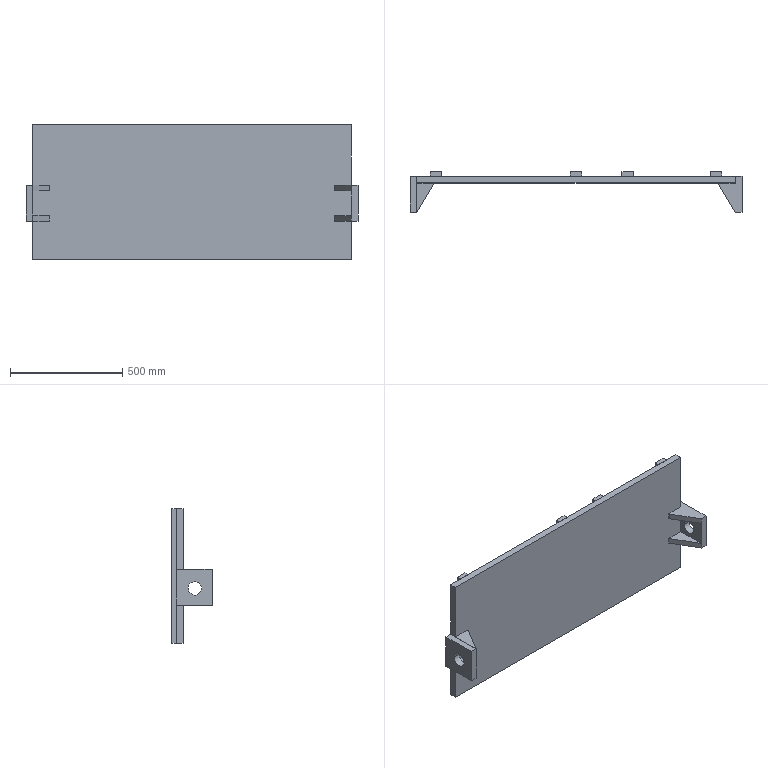Part | STEP file | PN_0001 Water tank base plate | 8 solids | 64 faces | box 1480 x 180 x 600 mm | volume 29823409 mm3 | plane 60 | cylinder 4 | commonest cylinder face diameters 60 x4